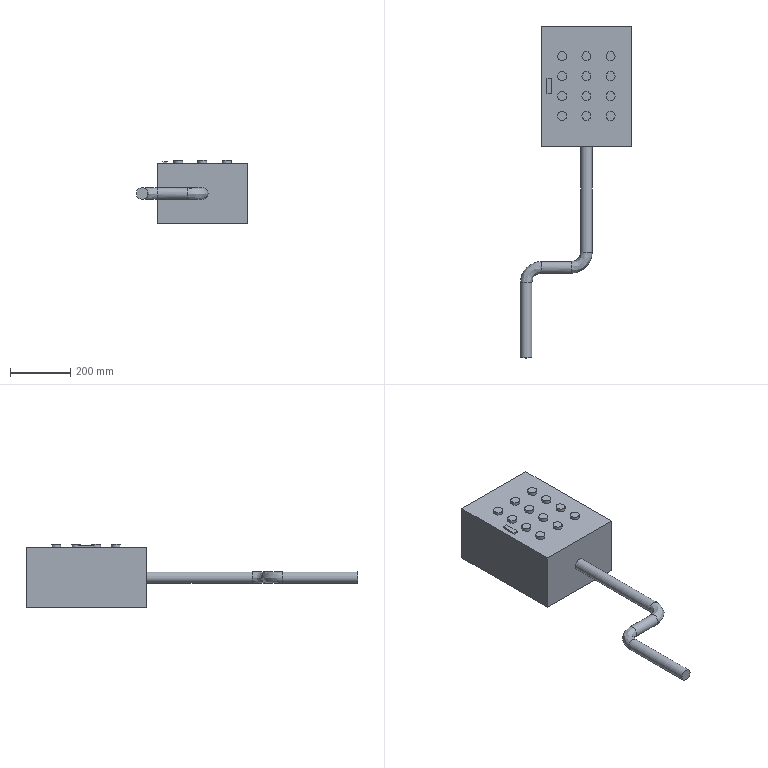Part | NX | features Panel 16 | 15 solids | 55 faces | box 369 x 1100 x 210 mm | volume 25060594 mm3 | plane 38 | cylinder 15 | spline 2 | commonest cylinder face diameters 30 x12 38 x3